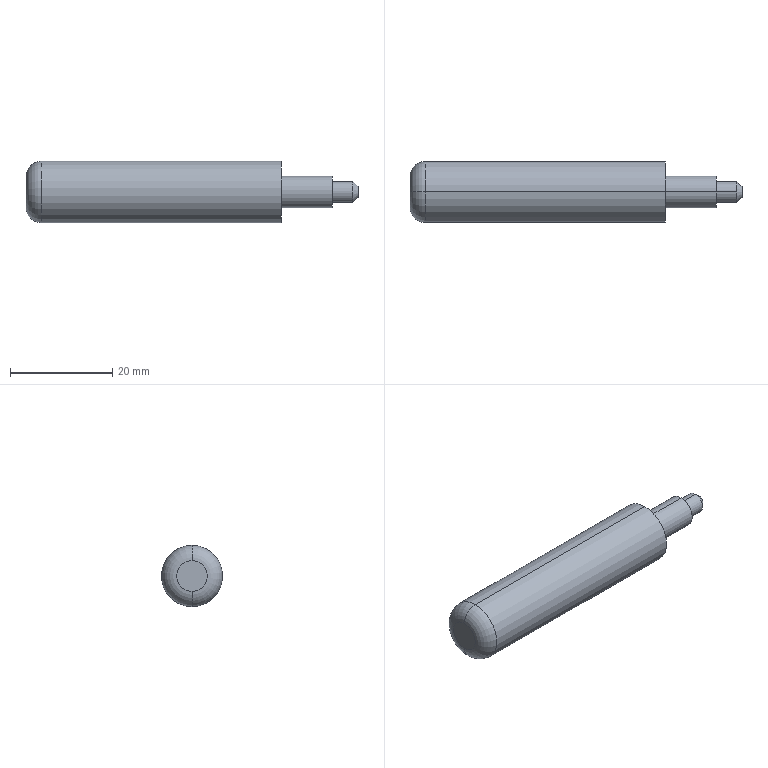Part | STEP file | Guide wheel mechanism revised.sldasm-Part-43 | 1 solid | 14 faces | box 65 x 12 x 12 mm | volume 5950 mm3 | cylinder 6 | plane 4 | torus 2 | cone 2 | commonest cylinder face diameters 4 x2 6.2 x2 12 x2
STEP:
#1=CARTESIAN_POINT('',(-50.,0.,3.));
#2=VERTEX_POINT('',#1);
#3=CARTESIAN_POINT('',(-50.,0.,-3.));
#4=VERTEX_POINT('',#3);
#5=CARTESIAN_POINT('',(-50.,0.,0.));
#6=DIRECTION('',(-1.,0.,0.));
#7=DIRECTION('',(0.,0.,-1.));
#8=AXIS2_PLACEMENT_3D('',#5,#6,#7);
#9=CIRCLE('',#8,3.);
#10=EDGE_CURVE('',#2,#4,#9,.T.);
#11=ORIENTED_EDGE('',*,*,#10,.F.);
#12=CARTESIAN_POINT('',(-47.,0.,6.));
#13=VERTEX_POINT('',#12);
#14=CARTESIAN_POINT('',(-47.,0.,3.));
#15=DIRECTION('',(0.,1.,0.));
#16=DIRECTION('',(0.,0.,1.));
#17=AXIS2_PLACEMENT_3D('',#14,#15,#16);
#18=CIRCLE('',#17,3.);
#19=EDGE_CURVE('',#2,#13,#18,.T.);
#20=ORIENTED_EDGE('',*,*,#19,.T.);
#21=CARTESIAN_POINT('',(-47.,0.,-6.));
#22=VERTEX_POINT('',#21);
#23=CARTESIAN_POINT('',(-47.,0.,0.));
#24=DIRECTION('',(1.,0.,0.));
#25=DIRECTION('',(0.,0.,-1.));
#26=AXIS2_PLACEMENT_3D('',#23,#24,#25);
#27=CIRCLE('',#26,6.);
#28=EDGE_CURVE('',#22,#13,#27,.T.);
#29=ORIENTED_EDGE('',*,*,#28,.F.);
#30=CARTESIAN_POINT('',(-47.,0.,-3.));
#31=DIRECTION('',(0.,-1.,0.));
#32=DIRECTION('',(0.,0.,-1.));
#33=AXIS2_PLACEMENT_3D('',#30,#31,#32);
#34=CIRCLE('',#33,3.);
#35=EDGE_CURVE('',#4,#22,#34,.T.);
#36=ORIENTED_EDGE('',*,*,#35,.F.);
#37=EDGE_LOOP('',(#11,#20,#29,#36));
#38=FACE_OUTER_BOUND('',#37,.T.);
#39=CARTESIAN_POINT('',(-47.,0.,0.));
#40=DIRECTION('',(1.,0.,0.));
#41=DIRECTION('',(0.,0.,-1.));
#42=AXIS2_PLACEMENT_3D('',#39,#40,#41);
#43=TOROIDAL_SURFACE('',#42,3.,3.);
#44=ADVANCED_FACE('',(#38),#43,.T.);
#45=CARTESIAN_POINT('',(15.,0.,1.));
#46=VERTEX_POINT('',#45);
#47=CARTESIAN_POINT('',(15.,0.,-1.));
#48=VERTEX_POINT('',#47);
#49=CARTESIAN_POINT('',(15.,0.,0.));
#50=DIRECTION('',(-1.,0.,0.));
#51=DIRECTION('',(0.,0.,1.));
#52=AXIS2_PLACEMENT_3D('',#49,#50,#51);
#53=CIRCLE('',#52,1.);
#54=EDGE_CURVE('',#46,#48,#53,.T.);
#55=ORIENTED_EDGE('',*,*,#54,.T.);
#56=CARTESIAN_POINT('',(14.,0.,-2.));
#57=VERTEX_POINT('',#56);
#58=CARTESIAN_POINT('',(15.,0.,-1.));
#59=DIRECTION('',(-0.7071,0.,-0.7071));
#60=VECTOR('',#59,1000.);
#61=LINE('',#58,#60);
#62=EDGE_CURVE('',#48,#57,#61,.T.);
#63=ORIENTED_EDGE('',*,*,#62,.T.);
#64=CARTESIAN_POINT('',(14.,0.,2.));
#65=VERTEX_POINT('',#64);
#66=CARTESIAN_POINT('',(14.,0.,0.));
#67=DIRECTION('',(-1.,0.,0.));
#68=DIRECTION('',(0.,0.,1.));
#69=AXIS2_PLACEMENT_3D('',#66,#67,#68);
#70=CIRCLE('',#69,2.);
#71=EDGE_CURVE('',#65,#57,#70,.T.);
#72=ORIENTED_EDGE('',*,*,#71,.F.);
#73=CARTESIAN_POINT('',(15.,0.,1.));
#74=DIRECTION('',(-0.7071,0.,0.7071));
#75=VECTOR('',#74,1000.);
#76=LINE('',#73,#75);
#77=EDGE_CURVE('',#46,#65,#76,.T.);
#78=ORIENTED_EDGE('',*,*,#77,.F.);
#79=EDGE_LOOP('',(#55,#63,#72,#78));
#80=FACE_OUTER_BOUND('',#79,.T.);
#81=CARTESIAN_POINT('',(15.,0.,0.));
#82=DIRECTION('',(-1.,0.,0.));
#83=DIRECTION('',(0.,0.,1.));
#84=AXIS2_PLACEMENT_3D('',#81,#82,#83);
#85=CONICAL_SURFACE('',#84,1.,0.7854);
#86=ADVANCED_FACE('',(#80),#85,.T.);
#87=ORIENTED_EDGE('',*,*,#71,.T.);
#88=CARTESIAN_POINT('',(10.,0.,-2.));
#89=VERTEX_POINT('',#88);
#90=CARTESIAN_POINT('',(15.,0.,-2.));
#91=DIRECTION('',(-1.,0.,0.));
#92=VECTOR('',#91,1000.);
#93=LINE('',#90,#92);
#94=EDGE_CURVE('',#57,#89,#93,.T.);
#95=ORIENTED_EDGE('',*,*,#94,.T.);
#96=CARTESIAN_POINT('',(10.,0.,2.));
#97=VERTEX_POINT('',#96);
#98=CARTESIAN_POINT('',(10.,0.,0.));
#99=DIRECTION('',(-1.,0.,0.));
#100=DIRECTION('',(0.,0.,1.));
#101=AXIS2_PLACEMENT_3D('',#98,#99,#100);
#102=CIRCLE('',#101,2.);
#103=EDGE_CURVE('',#97,#89,#102,.T.);
#104=ORIENTED_EDGE('',*,*,#103,.F.);
#105=CARTESIAN_POINT('',(15.,0.,2.));
#106=DIRECTION('',(-1.,0.,0.));
#107=VECTOR('',#106,1000.);
#108=LINE('',#105,#107);
#109=EDGE_CURVE('',#65,#97,#108,.T.);
#110=ORIENTED_EDGE('',*,*,#109,.F.);
#111=EDGE_LOOP('',(#87,#95,#104,#110));
#112=FACE_OUTER_BOUND('',#111,.T.);
#113=CARTESIAN_POINT('',(15.,0.,0.));
#114=DIRECTION('',(-1.,0.,0.));
#115=DIRECTION('',(0.,0.,1.));
#116=AXIS2_PLACEMENT_3D('',#113,#114,#115);
#117=CYLINDRICAL_SURFACE('',#116,2.);
#118=ADVANCED_FACE('',(#112),#117,.T.);
#119=CARTESIAN_POINT('',(10.,0.,3.1));
#120=VERTEX_POINT('',#119);
#121=CARTESIAN_POINT('',(10.,0.,-3.1));
#122=VERTEX_POINT('',#121);
#123=CARTESIAN_POINT('',(10.,0.,0.));
#124=DIRECTION('',(-1.,0.,0.));
#125=DIRECTION('',(0.,0.,1.));
#126=AXIS2_PLACEMENT_3D('',#123,#124,#125);
#127=CIRCLE('',#126,3.1);
#128=EDGE_CURVE('',#120,#122,#127,.T.);
#129=ORIENTED_EDGE('',*,*,#128,.T.);
#130=CARTESIAN_POINT('',(0.,0.,-3.1));
#131=VERTEX_POINT('',#130);
#132=CARTESIAN_POINT('',(15.,0.,-3.1));
#133=DIRECTION('',(-1.,0.,0.));
#134=VECTOR('',#133,1000.);
#135=LINE('',#132,#134);
#136=EDGE_CURVE('',#122,#131,#135,.T.);
#137=ORIENTED_EDGE('',*,*,#136,.T.);
#138=CARTESIAN_POINT('',(0.,0.,3.1));
#139=VERTEX_POINT('',#138);
#140=CARTESIAN_POINT('',(0.,0.,0.));
#141=DIRECTION('',(-1.,0.,0.));
#142=DIRECTION('',(0.,0.,1.));
#143=AXIS2_PLACEMENT_3D('',#140,#141,#142);
#144=CIRCLE('',#143,3.1);
#145=EDGE_CURVE('',#139,#131,#144,.T.);
#146=ORIENTED_EDGE('',*,*,#145,.F.);
#147=CARTESIAN_POINT('',(15.,0.,3.1));
#148=DIRECTION('',(-1.,0.,0.));
#149=VECTOR('',#148,1000.);
#150=LINE('',#147,#149);
#151=EDGE_CURVE('',#120,#139,#150,.T.);
#152=ORIENTED_EDGE('',*,*,#151,.F.);
#153=EDGE_LOOP('',(#129,#137,#146,#152));
#154=FACE_OUTER_BOUND('',#153,.T.);
#155=CARTESIAN_POINT('',(15.,0.,0.));
#156=DIRECTION('',(-1.,0.,0.));
#157=DIRECTION('',(0.,0.,1.));
#158=AXIS2_PLACEMENT_3D('',#155,#156,#157);
#159=CYLINDRICAL_SURFACE('',#158,3.1);
#160=ADVANCED_FACE('',(#154),#159,.T.);
#161=CARTESIAN_POINT('',(0.,0.,6.));
#162=VERTEX_POINT('',#161);
#163=CARTESIAN_POINT('',(0.,0.,-6.));
#164=VERTEX_POINT('',#163);
#165=CARTESIAN_POINT('',(0.,0.,0.));
#166=DIRECTION('',(-1.,0.,0.));
#167=DIRECTION('',(0.,0.,1.));
#168=AXIS2_PLACEMENT_3D('',#165,#166,#167);
#169=CIRCLE('',#168,6.);
#170=EDGE_CURVE('',#162,#164,#169,.T.);
#171=ORIENTED_EDGE('',*,*,#170,.T.);
#172=CARTESIAN_POINT('',(15.,0.,-6.));
#173=DIRECTION('',(-1.,0.,0.));
#174=VECTOR('',#173,1000.);
#175=LINE('',#172,#174);
#176=EDGE_CURVE('',#164,#22,#175,.T.);
#177=ORIENTED_EDGE('',*,*,#176,.T.);
#178=ORIENTED_EDGE('',*,*,#28,.T.);
#179=CARTESIAN_POINT('',(15.,0.,6.));
#180=DIRECTION('',(-1.,0.,0.));
#181=VECTOR('',#180,1000.);
#182=LINE('',#179,#181);
#183=EDGE_CURVE('',#162,#13,#182,.T.);
#184=ORIENTED_EDGE('',*,*,#183,.F.);
#185=EDGE_LOOP('',(#171,#177,#178,#184));
#186=FACE_OUTER_BOUND('',#185,.T.);
#187=CARTESIAN_POINT('',(15.,0.,0.));
#188=DIRECTION('',(-1.,0.,0.));
#189=DIRECTION('',(0.,0.,1.));
#190=AXIS2_PLACEMENT_3D('',#187,#188,#189);
#191=CYLINDRICAL_SURFACE('',#190,6.);
#192=ADVANCED_FACE('',(#186),#191,.T.);
#193=CARTESIAN_POINT('',(-50.,0.,0.));
#194=DIRECTION('',(-1.,0.,0.));
#195=DIRECTION('',(0.,0.,-1.));
#196=AXIS2_PLACEMENT_3D('',#193,#194,#195);
#197=CIRCLE('',#196,3.);
#198=EDGE_CURVE('',#4,#2,#197,.T.);
#199=ORIENTED_EDGE('',*,*,#198,.T.);
#200=ORIENTED_EDGE('',*,*,#10,.T.);
#201=EDGE_LOOP('',(#199,#200));
#202=FACE_OUTER_BOUND('',#201,.T.);
#203=CARTESIAN_POINT('',(-50.,0.,0.));
#204=DIRECTION('',(1.,0.,0.));
#205=DIRECTION('',(0.,0.,-1.));
#206=AXIS2_PLACEMENT_3D('',#203,#204,#205);
#207=PLANE('',#206);
#208=ADVANCED_FACE('',(#202),#207,.F.);
#209=ORIENTED_EDGE('',*,*,#176,.F.);
#210=CARTESIAN_POINT('',(0.,0.,0.));
#211=DIRECTION('',(-1.,0.,0.));
#212=DIRECTION('',(0.,0.,1.));
#213=AXIS2_PLACEMENT_3D('',#210,#211,#212);
#214=CIRCLE('',#213,6.);
#215=EDGE_CURVE('',#164,#162,#214,.T.);
#216=ORIENTED_EDGE('',*,*,#215,.T.);
#217=ORIENTED_EDGE('',*,*,#183,.T.);
#218=CARTESIAN_POINT('',(-47.,0.,0.));
#219=DIRECTION('',(1.,0.,0.));
#220=DIRECTION('',(0.,0.,-1.));
#221=AXIS2_PLACEMENT_3D('',#218,#219,#220);
#222=CIRCLE('',#221,6.);
#223=EDGE_CURVE('',#13,#22,#222,.T.);
#224=ORIENTED_EDGE('',*,*,#223,.T.);
#225=EDGE_LOOP('',(#209,#216,#217,#224));
#226=FACE_OUTER_BOUND('',#225,.T.);
#227=CARTESIAN_POINT('',(15.,0.,0.));
#228=DIRECTION('',(-1.,0.,0.));
#229=DIRECTION('',(0.,0.,1.));
#230=AXIS2_PLACEMENT_3D('',#227,#228,#229);
#231=CYLINDRICAL_SURFACE('',#230,6.);
#232=ADVANCED_FACE('',(#226),#231,.T.);
#233=ORIENTED_EDGE('',*,*,#170,.F.);
#234=ORIENTED_EDGE('',*,*,#215,.F.);
#235=EDGE_LOOP('',(#233,#234));
#236=FACE_OUTER_BOUND('',#235,.T.);
#237=ORIENTED_EDGE('',*,*,#145,.T.);
#238=CARTESIAN_POINT('',(0.,0.,0.));
#239=DIRECTION('',(-1.,0.,0.));
#240=DIRECTION('',(0.,0.,1.));
#241=AXIS2_PLACEMENT_3D('',#238,#239,#240);
#242=CIRCLE('',#241,3.1);
#243=EDGE_CURVE('',#131,#139,#242,.T.);
#244=ORIENTED_EDGE('',*,*,#243,.T.);
#245=EDGE_LOOP('',(#237,#244));
#246=FACE_BOUND('',#245,.T.);
#247=CARTESIAN_POINT('',(0.,6.,0.));
#248=DIRECTION('',(-1.,0.,0.));
#249=DIRECTION('',(0.,0.,1.));
#250=AXIS2_PLACEMENT_3D('',#247,#248,#249);
#251=PLANE('',#250);
#252=ADVANCED_FACE('',(#236,#246),#251,.F.);
#253=ORIENTED_EDGE('',*,*,#136,.F.);
#254=CARTESIAN_POINT('',(10.,0.,0.));
#255=DIRECTION('',(-1.,0.,0.));
#256=DIRECTION('',(0.,0.,1.));
#257=AXIS2_PLACEMENT_3D('',#254,#255,#256);
#258=CIRCLE('',#257,3.1);
#259=EDGE_CURVE('',#122,#120,#258,.T.);
#260=ORIENTED_EDGE('',*,*,#259,.T.);
#261=ORIENTED_EDGE('',*,*,#151,.T.);
#262=ORIENTED_EDGE('',*,*,#243,.F.);
#263=EDGE_LOOP('',(#253,#260,#261,#262));
#264=FACE_OUTER_BOUND('',#263,.T.);
#265=CARTESIAN_POINT('',(15.,0.,0.));
#266=DIRECTION('',(-1.,0.,0.));
#267=DIRECTION('',(0.,0.,1.));
#268=AXIS2_PLACEMENT_3D('',#265,#266,#267);
#269=CYLINDRICAL_SURFACE('',#268,3.1);
#270=ADVANCED_FACE('',(#264),#269,.T.);
#271=ORIENTED_EDGE('',*,*,#128,.F.);
#272=ORIENTED_EDGE('',*,*,#259,.F.);
#273=EDGE_LOOP('',(#271,#272));
#274=FACE_OUTER_BOUND('',#273,.T.);
#275=ORIENTED_EDGE('',*,*,#103,.T.);
#276=CARTESIAN_POINT('',(10.,0.,0.));
#277=DIRECTION('',(-1.,0.,0.));
#278=DIRECTION('',(0.,0.,1.));
#279=AXIS2_PLACEMENT_3D('',#276,#277,#278);
#280=CIRCLE('',#279,2.);
#281=EDGE_CURVE('',#89,#97,#280,.T.);
#282=ORIENTED_EDGE('',*,*,#281,.T.);
#283=EDGE_LOOP('',(#275,#282));
#284=FACE_BOUND('',#283,.T.);
#285=CARTESIAN_POINT('',(10.,3.1,0.));
#286=DIRECTION('',(-1.,0.,0.));
#287=DIRECTION('',(0.,0.,1.));
#288=AXIS2_PLACEMENT_3D('',#285,#286,#287);
#289=PLANE('',#288);
#290=ADVANCED_FACE('',(#274,#284),#289,.F.);
#291=ORIENTED_EDGE('',*,*,#94,.F.);
#292=CARTESIAN_POINT('',(14.,0.,0.));
#293=DIRECTION('',(-1.,0.,0.));
#294=DIRECTION('',(0.,0.,1.));
#295=AXIS2_PLACEMENT_3D('',#292,#293,#294);
#296=CIRCLE('',#295,2.);
#297=EDGE_CURVE('',#57,#65,#296,.T.);
#298=ORIENTED_EDGE('',*,*,#297,.T.);
#299=ORIENTED_EDGE('',*,*,#109,.T.);
#300=ORIENTED_EDGE('',*,*,#281,.F.);
#301=EDGE_LOOP('',(#291,#298,#299,#300));
#302=FACE_OUTER_BOUND('',#301,.T.);
#303=CARTESIAN_POINT('',(15.,0.,0.));
#304=DIRECTION('',(-1.,0.,0.));
#305=DIRECTION('',(0.,0.,1.));
#306=AXIS2_PLACEMENT_3D('',#303,#304,#305);
#307=CYLINDRICAL_SURFACE('',#306,2.);
#308=ADVANCED_FACE('',(#302),#307,.T.);
#309=ORIENTED_EDGE('',*,*,#62,.F.);
#310=CARTESIAN_POINT('',(15.,0.,0.));
#311=DIRECTION('',(-1.,0.,0.));
#312=DIRECTION('',(0.,0.,1.));
#313=AXIS2_PLACEMENT_3D('',#310,#311,#312);
#314=CIRCLE('',#313,1.);
#315=EDGE_CURVE('',#48,#46,#314,.T.);
#316=ORIENTED_EDGE('',*,*,#315,.T.);
#317=ORIENTED_EDGE('',*,*,#77,.T.);
#318=ORIENTED_EDGE('',*,*,#297,.F.);
#319=EDGE_LOOP('',(#309,#316,#317,#318));
#320=FACE_OUTER_BOUND('',#319,.T.);
#321=CARTESIAN_POINT('',(15.,0.,0.));
#322=DIRECTION('',(-1.,0.,0.));
#323=DIRECTION('',(0.,0.,1.));
#324=AXIS2_PLACEMENT_3D('',#321,#322,#323);
#325=CONICAL_SURFACE('',#324,1.,0.7854);
#326=ADVANCED_FACE('',(#320),#325,.T.);
#327=ORIENTED_EDGE('',*,*,#54,.F.);
#328=ORIENTED_EDGE('',*,*,#315,.F.);
#329=EDGE_LOOP('',(#327,#328));
#330=FACE_OUTER_BOUND('',#329,.T.);
#331=CARTESIAN_POINT('',(15.,1.,0.));
#332=DIRECTION('',(-1.,0.,0.));
#333=DIRECTION('',(0.,0.,1.));
#334=AXIS2_PLACEMENT_3D('',#331,#332,#333);
#335=PLANE('',#334);
#336=ADVANCED_FACE('',(#330),#335,.F.);
#337=ORIENTED_EDGE('',*,*,#19,.F.);
#338=ORIENTED_EDGE('',*,*,#198,.F.);
#339=ORIENTED_EDGE('',*,*,#35,.T.);
#340=ORIENTED_EDGE('',*,*,#223,.F.);
#341=EDGE_LOOP('',(#337,#338,#339,#340));
#342=FACE_OUTER_BOUND('',#341,.T.);
#343=CARTESIAN_POINT('',(-47.,0.,0.));
#344=DIRECTION('',(1.,0.,0.));
#345=DIRECTION('',(0.,0.,-1.));
#346=AXIS2_PLACEMENT_3D('',#343,#344,#345);
#347=TOROIDAL_SURFACE('',#346,3.,3.);
#348=ADVANCED_FACE('',(#342),#347,.T.);
#349=CLOSED_SHELL('',(#44,#86,#118,#160,#192,#208,#232,#252,#270,#290,#308,#326,#336,#348));
#350=MANIFOLD_SOLID_BREP('',#349);
#351=CARTESIAN_POINT('',(0.,0.,0.));
#352=DIRECTION('',(0.,0.,1.));
#353=DIRECTION('',(1.,0.,0.));
#354=AXIS2_PLACEMENT_3D('',#351,#352,#353);
#355=(LENGTH_UNIT()NAMED_UNIT(*)SI_UNIT(.MILLI.,.METRE.));
#356=UNCERTAINTY_MEASURE_WITH_UNIT(LENGTH_MEASURE(0.00001),#355,'','');
#357=(NAMED_UNIT(*)PLANE_ANGLE_UNIT()SI_UNIT($,.RADIAN.));
#358=(NAMED_UNIT(*)SI_UNIT($,.STERADIAN.)SOLID_ANGLE_UNIT());
#359=(GEOMETRIC_REPRESENTATION_CONTEXT(3)GLOBAL_UNCERTAINTY_ASSIGNED_CONTEXT((#356))GLOBAL_UNIT_ASSIGNED_CONTEXT((#355,#357,#358))REPRESENTATION_CONTEXT('',''));
#360=ADVANCED_BREP_SHAPE_REPRESENTATION('',(#350,#354),#359);